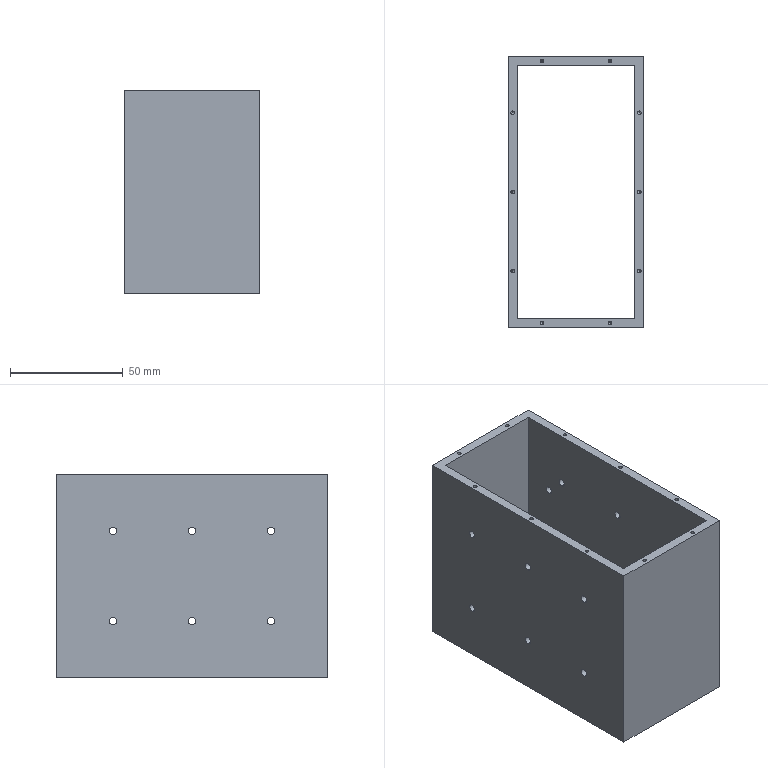Part | SolidWorks | features HoleWzd 4, Extrusion 1, Shell 1 | 1 solid | 130 faces | box 60 x 120 x 90 mm | volume 122991 mm3 | cylinder 72 | cone 48 | plane 10 | commonest cylinder face diameters 1.6 x40 3.3 x24 3.4 x8